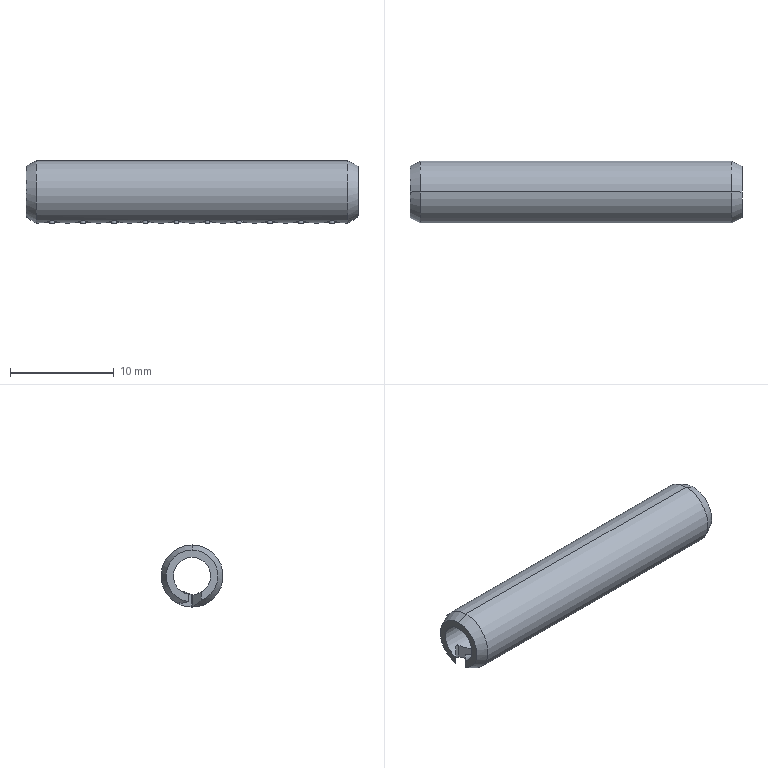Part | SolidWorks | features BaseBody 1 | 1 solid | 120 faces | box 32 x 6 x 6 mm | volume 521.254 mm3 | cylinder 68 | plane 46 | cone 6 | commonest cylinder face diameters 0.6 x42 3.6 x13 6 x13